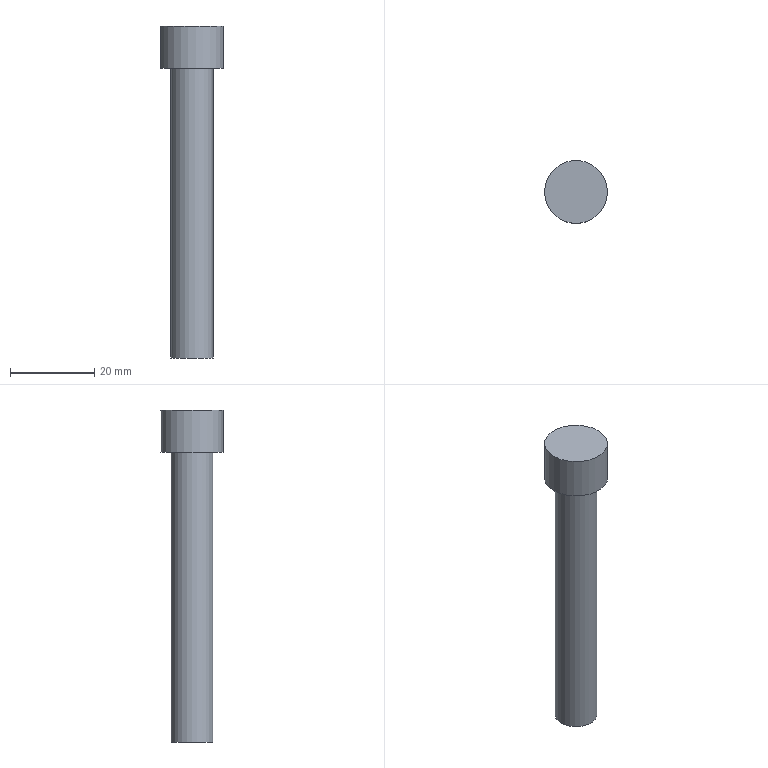Part | NX | features DATUM_CSYS 3, EXTRUDE 2, SKETCH 2, SYMBOLIC_THREAD 1 | 1 solid | 5 faces | box 15 x 15 x 79 mm | volume 7186 mm3 | plane 3 | cylinder 2 | commonest cylinder face diameters 10 x1 15 x1
STEP:
#1=CARTESIAN_POINT('',(5.,0.,0.));
#2=VERTEX_POINT('',#1);
#3=CARTESIAN_POINT('',(0.,0.,0.));
#4=DIRECTION('',(0.,0.,1.));
#5=DIRECTION('',(1.,0.,0.));
#6=AXIS2_PLACEMENT_3D('',#3,#4,#5);
#7=CIRCLE('',#6,5.);
#8=EDGE_CURVE('',#2,#2,#7,.T.);
#9=ORIENTED_EDGE('',*,*,#8,.T.);
#10=EDGE_LOOP('',(#9));
#11=FACE_BOUND('',#10,.T.);
#12=CARTESIAN_POINT('',(5.,0.,69.));
#13=VERTEX_POINT('',#12);
#14=CARTESIAN_POINT('',(0.,0.,69.));
#15=DIRECTION('',(0.,0.,1.));
#16=DIRECTION('',(1.,0.,0.));
#17=AXIS2_PLACEMENT_3D('',#14,#15,#16);
#18=CIRCLE('',#17,5.);
#19=EDGE_CURVE('',#13,#13,#18,.T.);
#20=ORIENTED_EDGE('',*,*,#19,.F.);
#21=EDGE_LOOP('',(#20));
#22=FACE_BOUND('',#21,.T.);
#23=CARTESIAN_POINT('',(0.,0.,79.));
#24=DIRECTION('',(0.,0.,-1.));
#25=DIRECTION('',(-1.,0.,0.));
#26=AXIS2_PLACEMENT_3D('',#23,#24,#25);
#27=CYLINDRICAL_SURFACE('',#26,5.);
#28=ADVANCED_FACE('',(#11,#22),#27,.T.);
#29=ORIENTED_EDGE('',*,*,#8,.F.);
#30=EDGE_LOOP('',(#29));
#31=FACE_BOUND('',#30,.T.);
#32=CARTESIAN_POINT('',(0.,0.,0.));
#33=DIRECTION('',(0.,0.,1.));
#34=DIRECTION('',(1.,0.,0.));
#35=AXIS2_PLACEMENT_3D('',#32,#33,#34);
#36=PLANE('',#35);
#37=ADVANCED_FACE('',(#31),#36,.F.);
#38=CARTESIAN_POINT('',(7.5,0.,69.));
#39=VERTEX_POINT('',#38);
#40=CARTESIAN_POINT('',(0.,0.,69.));
#41=DIRECTION('',(0.,0.,1.));
#42=DIRECTION('',(1.,0.,0.));
#43=AXIS2_PLACEMENT_3D('',#40,#41,#42);
#44=CIRCLE('',#43,7.5);
#45=EDGE_CURVE('',#39,#39,#44,.T.);
#46=ORIENTED_EDGE('',*,*,#45,.T.);
#47=EDGE_LOOP('',(#46));
#48=FACE_BOUND('',#47,.T.);
#49=CARTESIAN_POINT('',(7.5,0.,79.));
#50=VERTEX_POINT('',#49);
#51=CARTESIAN_POINT('',(0.,0.,79.));
#52=DIRECTION('',(0.,0.,1.));
#53=DIRECTION('',(1.,0.,0.));
#54=AXIS2_PLACEMENT_3D('',#51,#52,#53);
#55=CIRCLE('',#54,7.5);
#56=EDGE_CURVE('',#50,#50,#55,.T.);
#57=ORIENTED_EDGE('',*,*,#56,.F.);
#58=EDGE_LOOP('',(#57));
#59=FACE_BOUND('',#58,.T.);
#60=CARTESIAN_POINT('',(0.,0.,69.));
#61=DIRECTION('',(0.,0.,1.));
#62=DIRECTION('',(1.,0.,0.));
#63=AXIS2_PLACEMENT_3D('',#60,#61,#62);
#64=CYLINDRICAL_SURFACE('',#63,7.5);
#65=ADVANCED_FACE('',(#48,#59),#64,.T.);
#66=ORIENTED_EDGE('',*,*,#19,.T.);
#67=EDGE_LOOP('',(#66));
#68=FACE_BOUND('',#67,.T.);
#69=ORIENTED_EDGE('',*,*,#45,.F.);
#70=EDGE_LOOP('',(#69));
#71=FACE_BOUND('',#70,.T.);
#72=CARTESIAN_POINT('',(0.,0.,69.));
#73=DIRECTION('',(0.,0.,1.));
#74=DIRECTION('',(1.,0.,0.));
#75=AXIS2_PLACEMENT_3D('',#72,#73,#74);
#76=PLANE('',#75);
#77=ADVANCED_FACE('',(#68,#71),#76,.F.);
#78=ORIENTED_EDGE('',*,*,#56,.T.);
#79=EDGE_LOOP('',(#78));
#80=FACE_BOUND('',#79,.T.);
#81=CARTESIAN_POINT('',(0.,0.,79.));
#82=DIRECTION('',(0.,0.,1.));
#83=DIRECTION('',(1.,0.,0.));
#84=AXIS2_PLACEMENT_3D('',#81,#82,#83);
#85=PLANE('',#84);
#86=ADVANCED_FACE('',(#80),#85,.T.);
#87=CLOSED_SHELL('',(#28,#37,#65,#77,#86));
#88=MANIFOLD_SOLID_BREP('',#87);
#89=(LENGTH_UNIT()NAMED_UNIT(*)SI_UNIT(.MILLI.,.METRE.));
#90=UNCERTAINTY_MEASURE_WITH_UNIT(LENGTH_MEASURE(0.00001),#89,'','');
#91=(NAMED_UNIT(*)PLANE_ANGLE_UNIT()SI_UNIT($,.RADIAN.));
#92=(NAMED_UNIT(*)SI_UNIT($,.STERADIAN.)SOLID_ANGLE_UNIT());
#93=(GEOMETRIC_REPRESENTATION_CONTEXT(3)GLOBAL_UNCERTAINTY_ASSIGNED_CONTEXT((#90))GLOBAL_UNIT_ASSIGNED_CONTEXT((#89,#91,#92))REPRESENTATION_CONTEXT('',''));
#94=ADVANCED_BREP_SHAPE_REPRESENTATION('',(#88),#93);